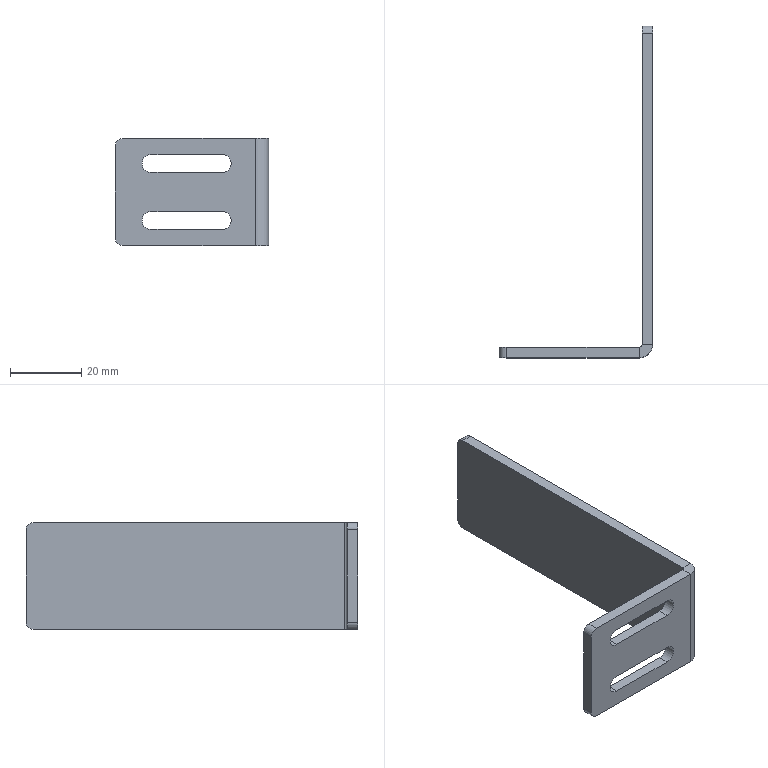Part | STEP file | ND25021-09-JDKM-03-BJ | 1 solid | 28 faces | box 43 x 93 x 30 mm | volume 11155 mm3 | plane 16 | cylinder 12 | commonest cylinder face diameters 5 x6 4 x4 1.473 x1 7.473 x1